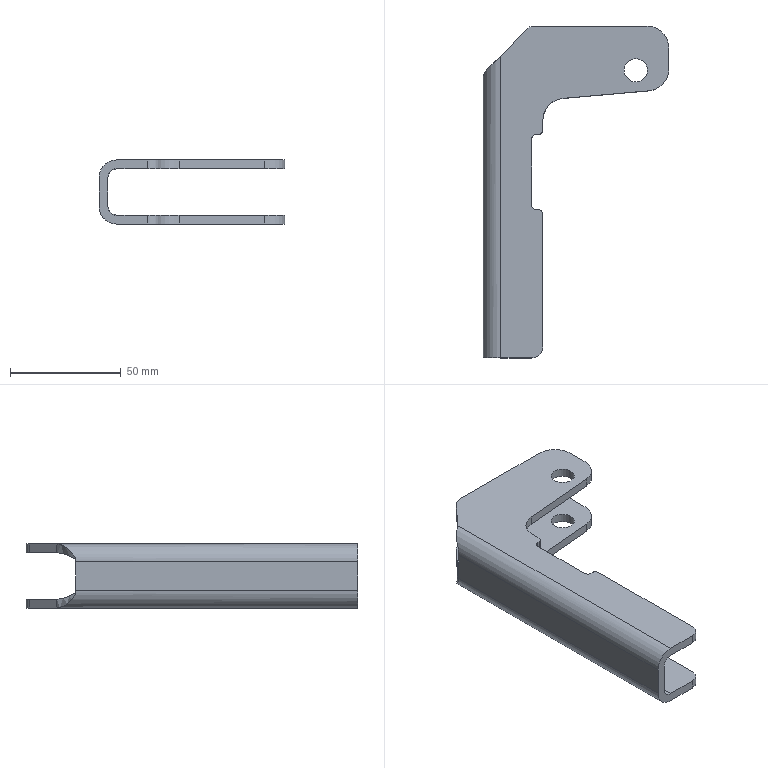Part | STEP file | Q7C0510 | 1 solid | 54 faces | box 84 x 150 x 29 mm | volume 50454 mm3 | plane 28 | cylinder 24 | spline 2 | commonest cylinder face diameters 4 x8 20 x6 10 x4 8 x2 10.5 x2 16 x2